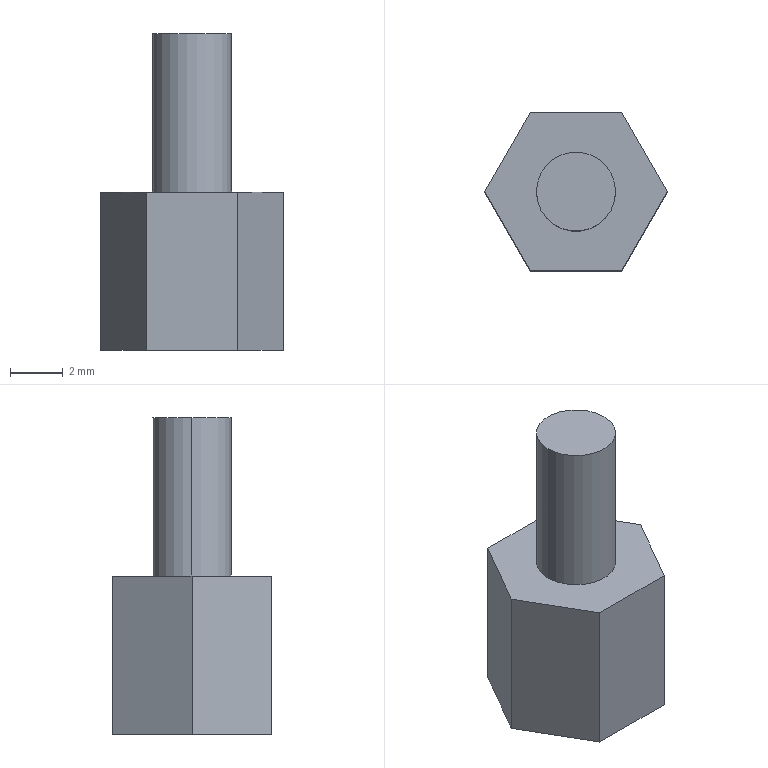Part | SolidWorks | features ICE 2, Extrusion 1 | 1 solid | 14 faces | box 6.928 x 6 x 12 mm | volume 208.267 mm3 | plane 10 | cylinder 4 | commonest cylinder face diameters 3 x4
STEP:
#1=CARTESIAN_POINT('',(1.5,0.,3.));
#2=VERTEX_POINT('',#1);
#3=CARTESIAN_POINT('',(-1.5,0.,3.));
#4=VERTEX_POINT('',#3);
#5=CARTESIAN_POINT('',(0.,0.,3.));
#6=DIRECTION('',(0.,0.,-1.));
#7=DIRECTION('',(-1.,0.,0.));
#8=AXIS2_PLACEMENT_3D('',#5,#6,#7);
#9=CIRCLE('',#8,1.5);
#10=EDGE_CURVE('',#2,#4,#9,.T.);
#11=ORIENTED_EDGE('',*,*,#10,.F.);
#12=CARTESIAN_POINT('',(1.5,0.,0.));
#13=VERTEX_POINT('',#12);
#14=CARTESIAN_POINT('',(1.5,0.,3.));
#15=DIRECTION('',(0.,0.,-1.));
#16=VECTOR('',#15,1000.);
#17=LINE('',#14,#16);
#18=EDGE_CURVE('',#2,#13,#17,.T.);
#19=ORIENTED_EDGE('',*,*,#18,.T.);
#20=CARTESIAN_POINT('',(-1.5,0.,0.));
#21=VERTEX_POINT('',#20);
#22=CARTESIAN_POINT('',(0.,0.,0.));
#23=DIRECTION('',(0.,0.,-1.));
#24=DIRECTION('',(-1.,0.,0.));
#25=AXIS2_PLACEMENT_3D('',#22,#23,#24);
#26=CIRCLE('',#25,1.5);
#27=EDGE_CURVE('',#13,#21,#26,.T.);
#28=ORIENTED_EDGE('',*,*,#27,.T.);
#29=CARTESIAN_POINT('',(-1.5,0.,3.));
#30=DIRECTION('',(0.,0.,-1.));
#31=VECTOR('',#30,1000.);
#32=LINE('',#29,#31);
#33=EDGE_CURVE('',#4,#21,#32,.T.);
#34=ORIENTED_EDGE('',*,*,#33,.F.);
#35=EDGE_LOOP('',(#11,#19,#28,#34));
#36=FACE_OUTER_BOUND('',#35,.T.);
#37=CARTESIAN_POINT('',(0.,0.,3.));
#38=DIRECTION('',(0.,0.,-1.));
#39=DIRECTION('',(-1.,0.,0.));
#40=AXIS2_PLACEMENT_3D('',#37,#38,#39);
#41=CYLINDRICAL_SURFACE('',#40,1.5);
#42=ADVANCED_FACE('',(#36),#41,.F.);
#43=CARTESIAN_POINT('',(1.5,0.,12.));
#44=VERTEX_POINT('',#43);
#45=CARTESIAN_POINT('',(-1.5,0.,12.));
#46=VERTEX_POINT('',#45);
#47=CARTESIAN_POINT('',(0.,0.,12.));
#48=DIRECTION('',(0.,0.,1.));
#49=DIRECTION('',(1.,0.,0.));
#50=AXIS2_PLACEMENT_3D('',#47,#48,#49);
#51=CIRCLE('',#50,1.5);
#52=EDGE_CURVE('',#44,#46,#51,.T.);
#53=ORIENTED_EDGE('',*,*,#52,.F.);
#54=CARTESIAN_POINT('',(1.5,0.,6.));
#55=VERTEX_POINT('',#54);
#56=CARTESIAN_POINT('',(1.5,0.,12.));
#57=DIRECTION('',(0.,0.,-1.));
#58=VECTOR('',#57,1000.);
#59=LINE('',#56,#58);
#60=EDGE_CURVE('',#44,#55,#59,.T.);
#61=ORIENTED_EDGE('',*,*,#60,.T.);
#62=CARTESIAN_POINT('',(-1.5,0.,6.));
#63=VERTEX_POINT('',#62);
#64=CARTESIAN_POINT('',(0.,0.,6.));
#65=DIRECTION('',(0.,0.,1.));
#66=DIRECTION('',(1.,0.,0.));
#67=AXIS2_PLACEMENT_3D('',#64,#65,#66);
#68=CIRCLE('',#67,1.5);
#69=EDGE_CURVE('',#55,#63,#68,.T.);
#70=ORIENTED_EDGE('',*,*,#69,.T.);
#71=CARTESIAN_POINT('',(-1.5,0.,12.));
#72=DIRECTION('',(0.,0.,-1.));
#73=VECTOR('',#72,1000.);
#74=LINE('',#71,#73);
#75=EDGE_CURVE('',#46,#63,#74,.T.);
#76=ORIENTED_EDGE('',*,*,#75,.F.);
#77=EDGE_LOOP('',(#53,#61,#70,#76));
#78=FACE_OUTER_BOUND('',#77,.T.);
#79=CARTESIAN_POINT('',(0.,0.,12.));
#80=DIRECTION('',(0.,0.,-1.));
#81=DIRECTION('',(-1.,0.,0.));
#82=AXIS2_PLACEMENT_3D('',#79,#80,#81);
#83=CYLINDRICAL_SURFACE('',#82,1.5);
#84=ADVANCED_FACE('',(#78),#83,.T.);
#85=CARTESIAN_POINT('',(1.732,-3.,0.));
#86=VERTEX_POINT('',#85);
#87=CARTESIAN_POINT('',(3.464,0.,0.));
#88=VERTEX_POINT('',#87);
#89=CARTESIAN_POINT('',(1.732,-3.,0.));
#90=DIRECTION('',(0.5,0.866,0.));
#91=VECTOR('',#90,1000.);
#92=LINE('',#89,#91);
#93=EDGE_CURVE('',#86,#88,#92,.T.);
#94=ORIENTED_EDGE('',*,*,#93,.T.);
#95=CARTESIAN_POINT('',(3.464,0.,6.));
#96=VERTEX_POINT('',#95);
#97=CARTESIAN_POINT('',(3.464,0.,6.));
#98=DIRECTION('',(0.,0.,-1.));
#99=VECTOR('',#98,1000.);
#100=LINE('',#97,#99);
#101=EDGE_CURVE('',#96,#88,#100,.T.);
#102=ORIENTED_EDGE('',*,*,#101,.F.);
#103=CARTESIAN_POINT('',(1.732,-3.,6.));
#104=VERTEX_POINT('',#103);
#105=CARTESIAN_POINT('',(1.732,-3.,6.));
#106=DIRECTION('',(0.5,0.866,0.));
#107=VECTOR('',#106,1000.);
#108=LINE('',#105,#107);
#109=EDGE_CURVE('',#104,#96,#108,.T.);
#110=ORIENTED_EDGE('',*,*,#109,.F.);
#111=CARTESIAN_POINT('',(1.732,-3.,6.));
#112=DIRECTION('',(0.,0.,-1.));
#113=VECTOR('',#112,1000.);
#114=LINE('',#111,#113);
#115=EDGE_CURVE('',#104,#86,#114,.T.);
#116=ORIENTED_EDGE('',*,*,#115,.T.);
#117=EDGE_LOOP('',(#94,#102,#110,#116));
#118=FACE_OUTER_BOUND('',#117,.T.);
#119=CARTESIAN_POINT('',(1.732,-3.,6.));
#120=DIRECTION('',(-0.866,0.5,0.));
#121=DIRECTION('',(-0.5,-0.866,0.));
#122=AXIS2_PLACEMENT_3D('',#119,#120,#121);
#123=PLANE('',#122);
#124=ADVANCED_FACE('',(#118),#123,.F.);
#125=CARTESIAN_POINT('',(1.732,3.,0.));
#126=VERTEX_POINT('',#125);
#127=CARTESIAN_POINT('',(3.464,0.,0.));
#128=DIRECTION('',(-0.5,0.866,0.));
#129=VECTOR('',#128,1000.);
#130=LINE('',#127,#129);
#131=EDGE_CURVE('',#88,#126,#130,.T.);
#132=ORIENTED_EDGE('',*,*,#131,.T.);
#133=CARTESIAN_POINT('',(1.732,3.,6.));
#134=VERTEX_POINT('',#133);
#135=CARTESIAN_POINT('',(1.732,3.,6.));
#136=DIRECTION('',(0.,0.,-1.));
#137=VECTOR('',#136,1000.);
#138=LINE('',#135,#137);
#139=EDGE_CURVE('',#134,#126,#138,.T.);
#140=ORIENTED_EDGE('',*,*,#139,.F.);
#141=CARTESIAN_POINT('',(3.464,0.,6.));
#142=DIRECTION('',(-0.5,0.866,0.));
#143=VECTOR('',#142,1000.);
#144=LINE('',#141,#143);
#145=EDGE_CURVE('',#96,#134,#144,.T.);
#146=ORIENTED_EDGE('',*,*,#145,.F.);
#147=ORIENTED_EDGE('',*,*,#101,.T.);
#148=EDGE_LOOP('',(#132,#140,#146,#147));
#149=FACE_OUTER_BOUND('',#148,.T.);
#150=CARTESIAN_POINT('',(3.464,0.,6.));
#151=DIRECTION('',(-0.866,-0.5,0.));
#152=DIRECTION('',(0.5,-0.866,0.));
#153=AXIS2_PLACEMENT_3D('',#150,#151,#152);
#154=PLANE('',#153);
#155=ADVANCED_FACE('',(#149),#154,.F.);
#156=CARTESIAN_POINT('',(-1.732,3.,0.));
#157=VERTEX_POINT('',#156);
#158=CARTESIAN_POINT('',(1.732,3.,0.));
#159=DIRECTION('',(-1.,0.,0.));
#160=VECTOR('',#159,1000.);
#161=LINE('',#158,#160);
#162=EDGE_CURVE('',#126,#157,#161,.T.);
#163=ORIENTED_EDGE('',*,*,#162,.T.);
#164=CARTESIAN_POINT('',(-1.732,3.,6.));
#165=VERTEX_POINT('',#164);
#166=CARTESIAN_POINT('',(-1.732,3.,6.));
#167=DIRECTION('',(0.,0.,-1.));
#168=VECTOR('',#167,1000.);
#169=LINE('',#166,#168);
#170=EDGE_CURVE('',#165,#157,#169,.T.);
#171=ORIENTED_EDGE('',*,*,#170,.F.);
#172=CARTESIAN_POINT('',(1.732,3.,6.));
#173=DIRECTION('',(-1.,0.,0.));
#174=VECTOR('',#173,1000.);
#175=LINE('',#172,#174);
#176=EDGE_CURVE('',#134,#165,#175,.T.);
#177=ORIENTED_EDGE('',*,*,#176,.F.);
#178=ORIENTED_EDGE('',*,*,#139,.T.);
#179=EDGE_LOOP('',(#163,#171,#177,#178));
#180=FACE_OUTER_BOUND('',#179,.T.);
#181=CARTESIAN_POINT('',(1.732,3.,6.));
#182=DIRECTION('',(0.,-1.,0.));
#183=DIRECTION('',(1.,0.,0.));
#184=AXIS2_PLACEMENT_3D('',#181,#182,#183);
#185=PLANE('',#184);
#186=ADVANCED_FACE('',(#180),#185,.F.);
#187=CARTESIAN_POINT('',(-3.464,0.,0.));
#188=VERTEX_POINT('',#187);
#189=CARTESIAN_POINT('',(-1.732,3.,0.));
#190=DIRECTION('',(-0.5,-0.866,0.));
#191=VECTOR('',#190,1000.);
#192=LINE('',#189,#191);
#193=EDGE_CURVE('',#157,#188,#192,.T.);
#194=ORIENTED_EDGE('',*,*,#193,.T.);
#195=CARTESIAN_POINT('',(-3.464,0.,6.));
#196=VERTEX_POINT('',#195);
#197=CARTESIAN_POINT('',(-3.464,0.,6.));
#198=DIRECTION('',(0.,0.,-1.));
#199=VECTOR('',#198,1000.);
#200=LINE('',#197,#199);
#201=EDGE_CURVE('',#196,#188,#200,.T.);
#202=ORIENTED_EDGE('',*,*,#201,.F.);
#203=CARTESIAN_POINT('',(-1.732,3.,6.));
#204=DIRECTION('',(-0.5,-0.866,0.));
#205=VECTOR('',#204,1000.);
#206=LINE('',#203,#205);
#207=EDGE_CURVE('',#165,#196,#206,.T.);
#208=ORIENTED_EDGE('',*,*,#207,.F.);
#209=ORIENTED_EDGE('',*,*,#170,.T.);
#210=EDGE_LOOP('',(#194,#202,#208,#209));
#211=FACE_OUTER_BOUND('',#210,.T.);
#212=CARTESIAN_POINT('',(-1.732,3.,6.));
#213=DIRECTION('',(0.866,-0.5,0.));
#214=DIRECTION('',(0.5,0.866,0.));
#215=AXIS2_PLACEMENT_3D('',#212,#213,#214);
#216=PLANE('',#215);
#217=ADVANCED_FACE('',(#211),#216,.F.);
#218=CARTESIAN_POINT('',(-1.732,-3.,0.));
#219=VERTEX_POINT('',#218);
#220=CARTESIAN_POINT('',(-3.464,0.,0.));
#221=DIRECTION('',(0.5,-0.866,0.));
#222=VECTOR('',#221,1000.);
#223=LINE('',#220,#222);
#224=EDGE_CURVE('',#188,#219,#223,.T.);
#225=ORIENTED_EDGE('',*,*,#224,.T.);
#226=CARTESIAN_POINT('',(-1.732,-3.,6.));
#227=VERTEX_POINT('',#226);
#228=CARTESIAN_POINT('',(-1.732,-3.,6.));
#229=DIRECTION('',(0.,0.,-1.));
#230=VECTOR('',#229,1000.);
#231=LINE('',#228,#230);
#232=EDGE_CURVE('',#227,#219,#231,.T.);
#233=ORIENTED_EDGE('',*,*,#232,.F.);
#234=CARTESIAN_POINT('',(-3.464,0.,6.));
#235=DIRECTION('',(0.5,-0.866,0.));
#236=VECTOR('',#235,1000.);
#237=LINE('',#234,#236);
#238=EDGE_CURVE('',#196,#227,#237,.T.);
#239=ORIENTED_EDGE('',*,*,#238,.F.);
#240=ORIENTED_EDGE('',*,*,#201,.T.);
#241=EDGE_LOOP('',(#225,#233,#239,#240));
#242=FACE_OUTER_BOUND('',#241,.T.);
#243=CARTESIAN_POINT('',(-3.464,0.,6.));
#244=DIRECTION('',(0.866,0.5,0.));
#245=DIRECTION('',(-0.5,0.866,0.));
#246=AXIS2_PLACEMENT_3D('',#243,#244,#245);
#247=PLANE('',#246);
#248=ADVANCED_FACE('',(#242),#247,.F.);
#249=CARTESIAN_POINT('',(-1.732,-3.,0.));
#250=DIRECTION('',(1.,0.,0.));
#251=VECTOR('',#250,1000.);
#252=LINE('',#249,#251);
#253=EDGE_CURVE('',#219,#86,#252,.T.);
#254=ORIENTED_EDGE('',*,*,#253,.T.);
#255=ORIENTED_EDGE('',*,*,#115,.F.);
#256=CARTESIAN_POINT('',(-1.732,-3.,6.));
#257=DIRECTION('',(1.,0.,0.));
#258=VECTOR('',#257,1000.);
#259=LINE('',#256,#258);
#260=EDGE_CURVE('',#227,#104,#259,.T.);
#261=ORIENTED_EDGE('',*,*,#260,.F.);
#262=ORIENTED_EDGE('',*,*,#232,.T.);
#263=EDGE_LOOP('',(#254,#255,#261,#262));
#264=FACE_OUTER_BOUND('',#263,.T.);
#265=CARTESIAN_POINT('',(-1.732,-3.,6.));
#266=DIRECTION('',(0.,1.,0.));
#267=DIRECTION('',(-1.,0.,0.));
#268=AXIS2_PLACEMENT_3D('',#265,#266,#267);
#269=PLANE('',#268);
#270=ADVANCED_FACE('',(#264),#269,.F.);
#271=CARTESIAN_POINT('',(0.,0.,6.));
#272=DIRECTION('',(0.,0.,1.));
#273=DIRECTION('',(1.,0.,0.));
#274=AXIS2_PLACEMENT_3D('',#271,#272,#273);
#275=CIRCLE('',#274,1.5);
#276=EDGE_CURVE('',#63,#55,#275,.T.);
#277=ORIENTED_EDGE('',*,*,#276,.F.);
#278=ORIENTED_EDGE('',*,*,#69,.F.);
#279=EDGE_LOOP('',(#277,#278));
#280=FACE_BOUND('',#279,.T.);
#281=ORIENTED_EDGE('',*,*,#109,.T.);
#282=ORIENTED_EDGE('',*,*,#145,.T.);
#283=ORIENTED_EDGE('',*,*,#176,.T.);
#284=ORIENTED_EDGE('',*,*,#207,.T.);
#285=ORIENTED_EDGE('',*,*,#238,.T.);
#286=ORIENTED_EDGE('',*,*,#260,.T.);
#287=EDGE_LOOP('',(#281,#282,#283,#284,#285,#286));
#288=FACE_OUTER_BOUND('',#287,.T.);
#289=CARTESIAN_POINT('',(0.,0.,6.));
#290=DIRECTION('',(0.,0.,1.));
#291=DIRECTION('',(1.,0.,0.));
#292=AXIS2_PLACEMENT_3D('',#289,#290,#291);
#293=PLANE('',#292);
#294=ADVANCED_FACE('',(#280,#288),#293,.T.);
#295=CARTESIAN_POINT('',(0.,0.,0.));
#296=DIRECTION('',(0.,0.,-1.));
#297=DIRECTION('',(-1.,0.,0.));
#298=AXIS2_PLACEMENT_3D('',#295,#296,#297);
#299=CIRCLE('',#298,1.5);
#300=EDGE_CURVE('',#21,#13,#299,.T.);
#301=ORIENTED_EDGE('',*,*,#300,.F.);
#302=ORIENTED_EDGE('',*,*,#27,.F.);
#303=EDGE_LOOP('',(#301,#302));
#304=FACE_BOUND('',#303,.T.);
#305=ORIENTED_EDGE('',*,*,#93,.F.);
#306=ORIENTED_EDGE('',*,*,#253,.F.);
#307=ORIENTED_EDGE('',*,*,#224,.F.);
#308=ORIENTED_EDGE('',*,*,#193,.F.);
#309=ORIENTED_EDGE('',*,*,#162,.F.);
#310=ORIENTED_EDGE('',*,*,#131,.F.);
#311=EDGE_LOOP('',(#305,#306,#307,#308,#309,#310));
#312=FACE_OUTER_BOUND('',#311,.T.);
#313=CARTESIAN_POINT('',(0.,0.,0.));
#314=DIRECTION('',(0.,0.,1.));
#315=DIRECTION('',(1.,0.,0.));
#316=AXIS2_PLACEMENT_3D('',#313,#314,#315);
#317=PLANE('',#316);
#318=ADVANCED_FACE('',(#304,#312),#317,.F.);
#319=ORIENTED_EDGE('',*,*,#60,.F.);
#320=CARTESIAN_POINT('',(0.,0.,12.));
#321=DIRECTION('',(0.,0.,1.));
#322=DIRECTION('',(1.,0.,0.));
#323=AXIS2_PLACEMENT_3D('',#320,#321,#322);
#324=CIRCLE('',#323,1.5);
#325=EDGE_CURVE('',#46,#44,#324,.T.);
#326=ORIENTED_EDGE('',*,*,#325,.F.);
#327=ORIENTED_EDGE('',*,*,#75,.T.);
#328=ORIENTED_EDGE('',*,*,#276,.T.);
#329=EDGE_LOOP('',(#319,#326,#327,#328));
#330=FACE_OUTER_BOUND('',#329,.T.);
#331=CARTESIAN_POINT('',(0.,0.,12.));
#332=DIRECTION('',(0.,0.,-1.));
#333=DIRECTION('',(-1.,0.,0.));
#334=AXIS2_PLACEMENT_3D('',#331,#332,#333);
#335=CYLINDRICAL_SURFACE('',#334,1.5);
#336=ADVANCED_FACE('',(#330),#335,.T.);
#337=ORIENTED_EDGE('',*,*,#325,.T.);
#338=ORIENTED_EDGE('',*,*,#52,.T.);
#339=EDGE_LOOP('',(#337,#338));
#340=FACE_OUTER_BOUND('',#339,.T.);
#341=CARTESIAN_POINT('',(0.,0.,12.));
#342=DIRECTION('',(0.,0.,1.));
#343=DIRECTION('',(1.,0.,0.));
#344=AXIS2_PLACEMENT_3D('',#341,#342,#343);
#345=PLANE('',#344);
#346=ADVANCED_FACE('',(#340),#345,.T.);
#347=ORIENTED_EDGE('',*,*,#18,.F.);
#348=CARTESIAN_POINT('',(0.,0.,3.));
#349=DIRECTION('',(0.,0.,-1.));
#350=DIRECTION('',(-1.,0.,0.));
#351=AXIS2_PLACEMENT_3D('',#348,#349,#350);
#352=CIRCLE('',#351,1.5);
#353=EDGE_CURVE('',#4,#2,#352,.T.);
#354=ORIENTED_EDGE('',*,*,#353,.F.);
#355=ORIENTED_EDGE('',*,*,#33,.T.);
#356=ORIENTED_EDGE('',*,*,#300,.T.);
#357=EDGE_LOOP('',(#347,#354,#355,#356));
#358=FACE_OUTER_BOUND('',#357,.T.);
#359=CARTESIAN_POINT('',(0.,0.,3.));
#360=DIRECTION('',(0.,0.,-1.));
#361=DIRECTION('',(-1.,0.,0.));
#362=AXIS2_PLACEMENT_3D('',#359,#360,#361);
#363=CYLINDRICAL_SURFACE('',#362,1.5);
#364=ADVANCED_FACE('',(#358),#363,.F.);
#365=ORIENTED_EDGE('',*,*,#353,.T.);
#366=ORIENTED_EDGE('',*,*,#10,.T.);
#367=EDGE_LOOP('',(#365,#366));
#368=FACE_OUTER_BOUND('',#367,.T.);
#369=CARTESIAN_POINT('',(0.,0.,3.));
#370=DIRECTION('',(0.,0.,-1.));
#371=DIRECTION('',(-1.,0.,0.));
#372=AXIS2_PLACEMENT_3D('',#369,#370,#371);
#373=PLANE('',#372);
#374=ADVANCED_FACE('',(#368),#373,.T.);
#375=CLOSED_SHELL('',(#42,#84,#124,#155,#186,#217,#248,#270,#294,#318,#336,#346,#364,#374));
#376=MANIFOLD_SOLID_BREP('',#375);
#377=CARTESIAN_POINT('',(0.,0.,0.));
#378=DIRECTION('',(0.,0.,1.));
#379=DIRECTION('',(1.,0.,0.));
#380=AXIS2_PLACEMENT_3D('',#377,#378,#379);
#381=(LENGTH_UNIT()NAMED_UNIT(*)SI_UNIT(.MILLI.,.METRE.));
#382=UNCERTAINTY_MEASURE_WITH_UNIT(LENGTH_MEASURE(0.00001),#381,'','');
#383=(NAMED_UNIT(*)PLANE_ANGLE_UNIT()SI_UNIT($,.RADIAN.));
#384=(NAMED_UNIT(*)SI_UNIT($,.STERADIAN.)SOLID_ANGLE_UNIT());
#385=(GEOMETRIC_REPRESENTATION_CONTEXT(3)GLOBAL_UNCERTAINTY_ASSIGNED_CONTEXT((#382))GLOBAL_UNIT_ASSIGNED_CONTEXT((#381,#383,#384))REPRESENTATION_CONTEXT('',''));
#386=ADVANCED_BREP_SHAPE_REPRESENTATION('',(#376,#380),#385);